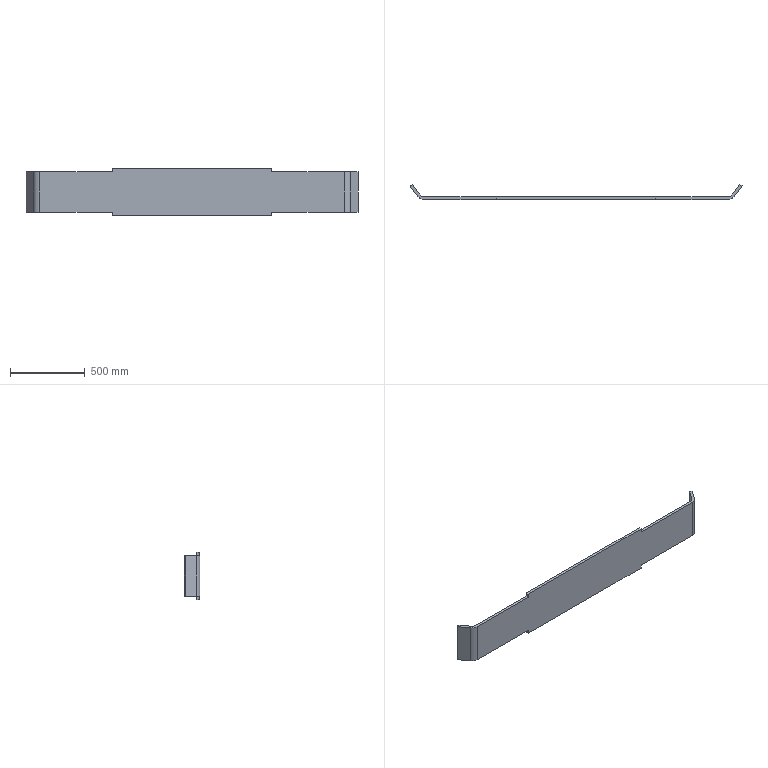Part | NX | features 前连杆 2 | 1 solid | 22 faces | box 2216 x 103.15 x 320 mm | volume 12312626 mm3 | plane 18 | cylinder 4 | commonest cylinder face diameters 60 x2 96.74 x2
STEP:
#1=CARTESIAN_POINT('',(-191.209,-83.211,25.));
#2=VERTEX_POINT('',#1);
#3=CARTESIAN_POINT('',(-243.821,-10.798,25.));
#4=VERTEX_POINT('',#3);
#5=CARTESIAN_POINT('',(957.045,-1663.648,25.));
#6=DIRECTION('',(-0.5878,0.809,0.));
#7=VECTOR('',#6,1000.);
#8=LINE('',#5,#7);
#9=EDGE_CURVE('',#2,#4,#8,.T.);
#10=ORIENTED_EDGE('',*,*,#9,.F.);
#11=CARTESIAN_POINT('',(-191.209,-83.211,295.));
#12=VERTEX_POINT('',#11);
#13=CARTESIAN_POINT('',(-191.209,-83.211,320.));
#14=DIRECTION('',(0.,0.,-1.));
#15=VECTOR('',#14,1000.);
#16=LINE('',#13,#15);
#17=EDGE_CURVE('',#12,#2,#16,.T.);
#18=ORIENTED_EDGE('',*,*,#17,.F.);
#19=CARTESIAN_POINT('',(-243.821,-10.798,295.));
#20=VERTEX_POINT('',#19);
#21=CARTESIAN_POINT('',(957.045,-1663.648,295.));
#22=DIRECTION('',(0.5878,-0.809,0.));
#23=VECTOR('',#22,1000.);
#24=LINE('',#21,#23);
#25=EDGE_CURVE('',#20,#12,#24,.T.);
#26=ORIENTED_EDGE('',*,*,#25,.F.);
#27=CARTESIAN_POINT('',(-243.821,-10.798,320.));
#28=DIRECTION('',(0.,0.,-1.));
#29=VECTOR('',#28,1000.);
#30=LINE('',#27,#29);
#31=EDGE_CURVE('',#20,#4,#30,.T.);
#32=ORIENTED_EDGE('',*,*,#31,.T.);
#33=EDGE_LOOP('',(#10,#18,#26,#32));
#34=FACE_BOUND('',#33,.T.);
#35=CARTESIAN_POINT('',(957.045,-1663.648,320.));
#36=DIRECTION('',(-0.809,-0.5878,0.));
#37=DIRECTION('',(0.5878,-0.809,0.));
#38=AXIS2_PLACEMENT_3D('',#35,#36,#37);
#39=PLANE('',#38);
#40=ADVANCED_FACE('',(#34),#39,.T.);
#41=ORIENTED_EDGE('',*,*,#17,.T.);
#42=CARTESIAN_POINT('',(-152.077,-103.15,25.));
#43=VERTEX_POINT('',#42);
#44=CARTESIAN_POINT('',(-152.077,-54.78,25.));
#45=DIRECTION('',(0.,0.,1.));
#46=DIRECTION('',(1.,0.,0.));
#47=AXIS2_PLACEMENT_3D('',#44,#45,#46);
#48=CIRCLE('',#47,48.37);
#49=EDGE_CURVE('',#2,#43,#48,.T.);
#50=ORIENTED_EDGE('',*,*,#49,.T.);
#51=CARTESIAN_POINT('',(-152.077,-103.15,295.));
#52=VERTEX_POINT('',#51);
#53=CARTESIAN_POINT('',(-152.077,-103.15,320.));
#54=DIRECTION('',(0.,0.,-1.));
#55=VECTOR('',#54,1000.);
#56=LINE('',#53,#55);
#57=EDGE_CURVE('',#52,#43,#56,.T.);
#58=ORIENTED_EDGE('',*,*,#57,.F.);
#59=CARTESIAN_POINT('',(-152.077,-54.78,295.));
#60=DIRECTION('',(0.,0.,-1.));
#61=DIRECTION('',(-1.,0.,0.));
#62=AXIS2_PLACEMENT_3D('',#59,#60,#61);
#63=CIRCLE('',#62,48.37);
#64=EDGE_CURVE('',#52,#12,#63,.T.);
#65=ORIENTED_EDGE('',*,*,#64,.T.);
#66=EDGE_LOOP('',(#41,#50,#58,#65));
#67=FACE_BOUND('',#66,.T.);
#68=CARTESIAN_POINT('',(-152.077,-54.78,320.));
#69=DIRECTION('',(0.,0.,-1.));
#70=DIRECTION('',(-1.,0.,0.));
#71=AXIS2_PLACEMENT_3D('',#68,#69,#70);
#72=CYLINDRICAL_SURFACE('',#71,48.37);
#73=ADVANCED_FACE('',(#67),#72,.T.);
#74=CARTESIAN_POINT('',(331.828,-103.15,25.));
#75=VERTEX_POINT('',#74);
#76=CARTESIAN_POINT('',(864.127,-103.15,25.));
#77=DIRECTION('',(1.,0.,0.));
#78=VECTOR('',#77,1000.);
#79=LINE('',#76,#78);
#80=EDGE_CURVE('',#43,#75,#79,.T.);
#81=ORIENTED_EDGE('',*,*,#80,.T.);
#82=CARTESIAN_POINT('',(331.828,-103.15,0.));
#83=VERTEX_POINT('',#82);
#84=CARTESIAN_POINT('',(331.828,-103.15,320.));
#85=DIRECTION('',(0.,0.,-1.));
#86=VECTOR('',#85,1000.);
#87=LINE('',#84,#86);
#88=EDGE_CURVE('',#75,#83,#87,.T.);
#89=ORIENTED_EDGE('',*,*,#88,.T.);
#90=CARTESIAN_POINT('',(1396.426,-103.15,0.));
#91=VERTEX_POINT('',#90);
#92=CARTESIAN_POINT('',(864.127,-103.15,0.));
#93=DIRECTION('',(1.,0.,0.));
#94=VECTOR('',#93,1000.);
#95=LINE('',#92,#94);
#96=EDGE_CURVE('',#83,#91,#95,.T.);
#97=ORIENTED_EDGE('',*,*,#96,.T.);
#98=CARTESIAN_POINT('',(1396.426,-103.15,25.));
#99=VERTEX_POINT('',#98);
#100=CARTESIAN_POINT('',(1396.426,-103.15,320.));
#101=DIRECTION('',(0.,0.,1.));
#102=VECTOR('',#101,1000.);
#103=LINE('',#100,#102);
#104=EDGE_CURVE('',#91,#99,#103,.T.);
#105=ORIENTED_EDGE('',*,*,#104,.T.);
#106=CARTESIAN_POINT('',(1880.331,-103.15,25.));
#107=VERTEX_POINT('',#106);
#108=CARTESIAN_POINT('',(864.127,-103.15,25.));
#109=DIRECTION('',(1.,0.,0.));
#110=VECTOR('',#109,1000.);
#111=LINE('',#108,#110);
#112=EDGE_CURVE('',#99,#107,#111,.T.);
#113=ORIENTED_EDGE('',*,*,#112,.T.);
#114=CARTESIAN_POINT('',(1880.331,-103.15,295.));
#115=VERTEX_POINT('',#114);
#116=CARTESIAN_POINT('',(1880.331,-103.15,320.));
#117=DIRECTION('',(0.,0.,-1.));
#118=VECTOR('',#117,1000.);
#119=LINE('',#116,#118);
#120=EDGE_CURVE('',#115,#107,#119,.T.);
#121=ORIENTED_EDGE('',*,*,#120,.F.);
#122=CARTESIAN_POINT('',(1396.426,-103.15,295.));
#123=VERTEX_POINT('',#122);
#124=CARTESIAN_POINT('',(864.127,-103.15,295.));
#125=DIRECTION('',(-1.,0.,0.));
#126=VECTOR('',#125,1000.);
#127=LINE('',#124,#126);
#128=EDGE_CURVE('',#115,#123,#127,.T.);
#129=ORIENTED_EDGE('',*,*,#128,.T.);
#130=CARTESIAN_POINT('',(1396.426,-103.15,320.));
#131=VERTEX_POINT('',#130);
#132=CARTESIAN_POINT('',(1396.426,-103.15,320.));
#133=DIRECTION('',(0.,0.,1.));
#134=VECTOR('',#133,1000.);
#135=LINE('',#132,#134);
#136=EDGE_CURVE('',#123,#131,#135,.T.);
#137=ORIENTED_EDGE('',*,*,#136,.T.);
#138=CARTESIAN_POINT('',(331.828,-103.15,320.));
#139=VERTEX_POINT('',#138);
#140=CARTESIAN_POINT('',(864.127,-103.15,320.));
#141=DIRECTION('',(1.,0.,0.));
#142=VECTOR('',#141,1000.);
#143=LINE('',#140,#142);
#144=EDGE_CURVE('',#139,#131,#143,.T.);
#145=ORIENTED_EDGE('',*,*,#144,.F.);
#146=CARTESIAN_POINT('',(331.828,-103.15,295.));
#147=VERTEX_POINT('',#146);
#148=CARTESIAN_POINT('',(331.828,-103.15,320.));
#149=DIRECTION('',(0.,0.,-1.));
#150=VECTOR('',#149,1000.);
#151=LINE('',#148,#150);
#152=EDGE_CURVE('',#139,#147,#151,.T.);
#153=ORIENTED_EDGE('',*,*,#152,.T.);
#154=CARTESIAN_POINT('',(864.127,-103.15,295.));
#155=DIRECTION('',(-1.,0.,0.));
#156=VECTOR('',#155,1000.);
#157=LINE('',#154,#156);
#158=EDGE_CURVE('',#147,#52,#157,.T.);
#159=ORIENTED_EDGE('',*,*,#158,.T.);
#160=ORIENTED_EDGE('',*,*,#57,.T.);
#161=EDGE_LOOP('',(#81,#89,#97,#105,#113,#121,#129,#137,#145,#153,#159,#160));
#162=FACE_BOUND('',#161,.T.);
#163=CARTESIAN_POINT('',(864.127,-103.15,320.));
#164=DIRECTION('',(0.,1.,0.));
#165=DIRECTION('',(-1.,0.,0.));
#166=AXIS2_PLACEMENT_3D('',#163,#164,#165);
#167=PLANE('',#166);
#168=ADVANCED_FACE('',(#162),#167,.F.);
#169=CARTESIAN_POINT('',(1919.464,-83.211,25.));
#170=VERTEX_POINT('',#169);
#171=CARTESIAN_POINT('',(1880.331,-54.78,25.));
#172=DIRECTION('',(0.,0.,1.));
#173=DIRECTION('',(1.,0.,0.));
#174=AXIS2_PLACEMENT_3D('',#171,#172,#173);
#175=CIRCLE('',#174,48.37);
#176=EDGE_CURVE('',#170,#107,#175,.F.);
#177=ORIENTED_EDGE('',*,*,#176,.F.);
#178=CARTESIAN_POINT('',(1919.464,-83.211,295.));
#179=VERTEX_POINT('',#178);
#180=CARTESIAN_POINT('',(1919.464,-83.211,320.));
#181=DIRECTION('',(0.,0.,-1.));
#182=VECTOR('',#181,1000.);
#183=LINE('',#180,#182);
#184=EDGE_CURVE('',#179,#170,#183,.T.);
#185=ORIENTED_EDGE('',*,*,#184,.F.);
#186=CARTESIAN_POINT('',(1880.331,-54.78,295.));
#187=DIRECTION('',(0.,0.,-1.));
#188=DIRECTION('',(-1.,0.,0.));
#189=AXIS2_PLACEMENT_3D('',#186,#187,#188);
#190=CIRCLE('',#189,48.37);
#191=EDGE_CURVE('',#115,#179,#190,.F.);
#192=ORIENTED_EDGE('',*,*,#191,.F.);
#193=ORIENTED_EDGE('',*,*,#120,.T.);
#194=EDGE_LOOP('',(#177,#185,#192,#193));
#195=FACE_BOUND('',#194,.T.);
#196=CARTESIAN_POINT('',(1880.331,-54.78,320.));
#197=DIRECTION('',(0.,0.,-1.));
#198=DIRECTION('',(-1.,0.,0.));
#199=AXIS2_PLACEMENT_3D('',#196,#197,#198);
#200=CYLINDRICAL_SURFACE('',#199,48.37);
#201=ADVANCED_FACE('',(#195),#200,.T.);
#202=ORIENTED_EDGE('',*,*,#184,.T.);
#203=CARTESIAN_POINT('',(1972.075,-10.798,25.));
#204=VERTEX_POINT('',#203);
#205=CARTESIAN_POINT('',(771.209,-1663.648,25.));
#206=DIRECTION('',(0.5878,0.809,0.));
#207=VECTOR('',#206,1000.);
#208=LINE('',#205,#207);
#209=EDGE_CURVE('',#170,#204,#208,.T.);
#210=ORIENTED_EDGE('',*,*,#209,.T.);
#211=CARTESIAN_POINT('',(1972.075,-10.798,295.));
#212=VERTEX_POINT('',#211);
#213=CARTESIAN_POINT('',(1972.075,-10.798,320.));
#214=DIRECTION('',(0.,0.,-1.));
#215=VECTOR('',#214,1000.);
#216=LINE('',#213,#215);
#217=EDGE_CURVE('',#212,#204,#216,.T.);
#218=ORIENTED_EDGE('',*,*,#217,.F.);
#219=CARTESIAN_POINT('',(771.209,-1663.648,295.));
#220=DIRECTION('',(-0.5878,-0.809,0.));
#221=VECTOR('',#220,1000.);
#222=LINE('',#219,#221);
#223=EDGE_CURVE('',#212,#179,#222,.T.);
#224=ORIENTED_EDGE('',*,*,#223,.T.);
#225=EDGE_LOOP('',(#202,#210,#218,#224));
#226=FACE_BOUND('',#225,.T.);
#227=CARTESIAN_POINT('',(771.209,-1663.648,320.));
#228=DIRECTION('',(-0.809,0.5878,0.));
#229=DIRECTION('',(-0.5878,-0.809,0.));
#230=AXIS2_PLACEMENT_3D('',#227,#228,#229);
#231=PLANE('',#230);
#232=ADVANCED_FACE('',(#226),#231,.F.);
#233=ORIENTED_EDGE('',*,*,#217,.T.);
#234=CARTESIAN_POINT('',(1957.213,0.,25.));
#235=VERTEX_POINT('',#234);
#236=CARTESIAN_POINT('',(2064.993,-78.307,25.));
#237=DIRECTION('',(-0.809,0.5878,0.));
#238=VECTOR('',#237,1000.);
#239=LINE('',#236,#238);
#240=EDGE_CURVE('',#204,#235,#239,.T.);
#241=ORIENTED_EDGE('',*,*,#240,.T.);
#242=CARTESIAN_POINT('',(1957.213,0.,295.));
#243=VERTEX_POINT('',#242);
#244=CARTESIAN_POINT('',(1957.213,0.,320.));
#245=DIRECTION('',(0.,0.,-1.));
#246=VECTOR('',#245,1000.);
#247=LINE('',#244,#246);
#248=EDGE_CURVE('',#243,#235,#247,.T.);
#249=ORIENTED_EDGE('',*,*,#248,.F.);
#250=CARTESIAN_POINT('',(2064.993,-78.307,295.));
#251=DIRECTION('',(0.809,-0.5878,0.));
#252=VECTOR('',#251,1000.);
#253=LINE('',#250,#252);
#254=EDGE_CURVE('',#243,#212,#253,.T.);
#255=ORIENTED_EDGE('',*,*,#254,.T.);
#256=EDGE_LOOP('',(#233,#241,#249,#255));
#257=FACE_BOUND('',#256,.T.);
#258=CARTESIAN_POINT('',(2064.993,-78.307,320.));
#259=DIRECTION('',(-0.5878,-0.809,0.));
#260=DIRECTION('',(0.809,-0.5878,0.));
#261=AXIS2_PLACEMENT_3D('',#258,#259,#260);
#262=PLANE('',#261);
#263=ADVANCED_FACE('',(#257),#262,.F.);
#264=CARTESIAN_POINT('',(1904.602,-72.414,25.));
#265=VERTEX_POINT('',#264);
#266=CARTESIAN_POINT('',(756.347,-1652.851,25.));
#267=DIRECTION('',(0.5878,0.809,0.));
#268=VECTOR('',#267,1000.);
#269=LINE('',#266,#268);
#270=EDGE_CURVE('',#265,#235,#269,.T.);
#271=ORIENTED_EDGE('',*,*,#270,.F.);
#272=CARTESIAN_POINT('',(1904.602,-72.414,295.));
#273=VERTEX_POINT('',#272);
#274=CARTESIAN_POINT('',(1904.602,-72.414,320.));
#275=DIRECTION('',(0.,0.,-1.));
#276=VECTOR('',#275,1000.);
#277=LINE('',#274,#276);
#278=EDGE_CURVE('',#273,#265,#277,.T.);
#279=ORIENTED_EDGE('',*,*,#278,.F.);
#280=CARTESIAN_POINT('',(756.347,-1652.851,295.));
#281=DIRECTION('',(-0.5878,-0.809,0.));
#282=VECTOR('',#281,1000.);
#283=LINE('',#280,#282);
#284=EDGE_CURVE('',#243,#273,#283,.T.);
#285=ORIENTED_EDGE('',*,*,#284,.F.);
#286=ORIENTED_EDGE('',*,*,#248,.T.);
#287=EDGE_LOOP('',(#271,#279,#285,#286));
#288=FACE_BOUND('',#287,.T.);
#289=CARTESIAN_POINT('',(756.347,-1652.851,320.));
#290=DIRECTION('',(-0.809,0.5878,0.));
#291=DIRECTION('',(-0.5878,-0.809,0.));
#292=AXIS2_PLACEMENT_3D('',#289,#290,#291);
#293=PLANE('',#292);
#294=ADVANCED_FACE('',(#288),#293,.T.);
#295=ORIENTED_EDGE('',*,*,#278,.T.);
#296=CARTESIAN_POINT('',(1880.331,-84.78,25.));
#297=VERTEX_POINT('',#296);
#298=CARTESIAN_POINT('',(1880.331,-54.78,25.));
#299=DIRECTION('',(0.,0.,1.));
#300=DIRECTION('',(1.,0.,0.));
#301=AXIS2_PLACEMENT_3D('',#298,#299,#300);
#302=CIRCLE('',#301,30.);
#303=EDGE_CURVE('',#265,#297,#302,.F.);
#304=ORIENTED_EDGE('',*,*,#303,.T.);
#305=CARTESIAN_POINT('',(1880.331,-84.78,295.));
#306=VERTEX_POINT('',#305);
#307=CARTESIAN_POINT('',(1880.331,-84.78,320.));
#308=DIRECTION('',(0.,0.,-1.));
#309=VECTOR('',#308,1000.);
#310=LINE('',#307,#309);
#311=EDGE_CURVE('',#306,#297,#310,.T.);
#312=ORIENTED_EDGE('',*,*,#311,.F.);
#313=CARTESIAN_POINT('',(1880.331,-54.78,295.));
#314=DIRECTION('',(0.,0.,-1.));
#315=DIRECTION('',(-1.,0.,0.));
#316=AXIS2_PLACEMENT_3D('',#313,#314,#315);
#317=CIRCLE('',#316,30.);
#318=EDGE_CURVE('',#306,#273,#317,.F.);
#319=ORIENTED_EDGE('',*,*,#318,.T.);
#320=EDGE_LOOP('',(#295,#304,#312,#319));
#321=FACE_BOUND('',#320,.T.);
#322=CARTESIAN_POINT('',(1880.331,-54.78,320.));
#323=DIRECTION('',(0.,0.,-1.));
#324=DIRECTION('',(-1.,0.,0.));
#325=AXIS2_PLACEMENT_3D('',#322,#323,#324);
#326=CYLINDRICAL_SURFACE('',#325,30.);
#327=ADVANCED_FACE('',(#321),#326,.F.);
#328=CARTESIAN_POINT('',(331.828,-84.78,25.));
#329=VERTEX_POINT('',#328);
#330=CARTESIAN_POINT('',(331.828,-84.78,0.));
#331=VERTEX_POINT('',#330);
#332=CARTESIAN_POINT('',(331.828,-84.78,320.));
#333=DIRECTION('',(0.,0.,-1.));
#334=VECTOR('',#333,1000.);
#335=LINE('',#332,#334);
#336=EDGE_CURVE('',#329,#331,#335,.T.);
#337=ORIENTED_EDGE('',*,*,#336,.F.);
#338=CARTESIAN_POINT('',(-152.077,-84.78,25.));
#339=VERTEX_POINT('',#338);
#340=CARTESIAN_POINT('',(864.127,-84.78,25.));
#341=DIRECTION('',(1.,0.,0.));
#342=VECTOR('',#341,1000.);
#343=LINE('',#340,#342);
#344=EDGE_CURVE('',#339,#329,#343,.T.);
#345=ORIENTED_EDGE('',*,*,#344,.F.);
#346=CARTESIAN_POINT('',(-152.077,-84.78,295.));
#347=VERTEX_POINT('',#346);
#348=CARTESIAN_POINT('',(-152.077,-84.78,320.));
#349=DIRECTION('',(0.,0.,-1.));
#350=VECTOR('',#349,1000.);
#351=LINE('',#348,#350);
#352=EDGE_CURVE('',#347,#339,#351,.T.);
#353=ORIENTED_EDGE('',*,*,#352,.F.);
#354=CARTESIAN_POINT('',(331.828,-84.78,295.));
#355=VERTEX_POINT('',#354);
#356=CARTESIAN_POINT('',(864.127,-84.78,295.));
#357=DIRECTION('',(-1.,0.,0.));
#358=VECTOR('',#357,1000.);
#359=LINE('',#356,#358);
#360=EDGE_CURVE('',#355,#347,#359,.T.);
#361=ORIENTED_EDGE('',*,*,#360,.F.);
#362=CARTESIAN_POINT('',(331.828,-84.78,320.));
#363=VERTEX_POINT('',#362);
#364=CARTESIAN_POINT('',(331.828,-84.78,320.));
#365=DIRECTION('',(0.,0.,-1.));
#366=VECTOR('',#365,1000.);
#367=LINE('',#364,#366);
#368=EDGE_CURVE('',#363,#355,#367,.T.);
#369=ORIENTED_EDGE('',*,*,#368,.F.);
#370=CARTESIAN_POINT('',(1396.426,-84.78,320.));
#371=VERTEX_POINT('',#370);
#372=CARTESIAN_POINT('',(864.127,-84.78,320.));
#373=DIRECTION('',(1.,0.,0.));
#374=VECTOR('',#373,1000.);
#375=LINE('',#372,#374);
#376=EDGE_CURVE('',#363,#371,#375,.T.);
#377=ORIENTED_EDGE('',*,*,#376,.T.);
#378=CARTESIAN_POINT('',(1396.426,-84.78,295.));
#379=VERTEX_POINT('',#378);
#380=CARTESIAN_POINT('',(1396.426,-84.78,320.));
#381=DIRECTION('',(0.,0.,1.));
#382=VECTOR('',#381,1000.);
#383=LINE('',#380,#382);
#384=EDGE_CURVE('',#379,#371,#383,.T.);
#385=ORIENTED_EDGE('',*,*,#384,.F.);
#386=CARTESIAN_POINT('',(864.127,-84.78,295.));
#387=DIRECTION('',(-1.,0.,0.));
#388=VECTOR('',#387,1000.);
#389=LINE('',#386,#388);
#390=EDGE_CURVE('',#306,#379,#389,.T.);
#391=ORIENTED_EDGE('',*,*,#390,.F.);
#392=ORIENTED_EDGE('',*,*,#311,.T.);
#393=CARTESIAN_POINT('',(1396.426,-84.78,25.));
#394=VERTEX_POINT('',#393);
#395=CARTESIAN_POINT('',(864.127,-84.78,25.));
#396=DIRECTION('',(1.,0.,0.));
#397=VECTOR('',#396,1000.);
#398=LINE('',#395,#397);
#399=EDGE_CURVE('',#394,#297,#398,.T.);
#400=ORIENTED_EDGE('',*,*,#399,.F.);
#401=CARTESIAN_POINT('',(1396.426,-84.78,0.));
#402=VERTEX_POINT('',#401);
#403=CARTESIAN_POINT('',(1396.426,-84.78,320.));
#404=DIRECTION('',(0.,0.,1.));
#405=VECTOR('',#404,1000.);
#406=LINE('',#403,#405);
#407=EDGE_CURVE('',#402,#394,#406,.T.);
#408=ORIENTED_EDGE('',*,*,#407,.F.);
#409=CARTESIAN_POINT('',(864.127,-84.78,0.));
#410=DIRECTION('',(1.,0.,0.));
#411=VECTOR('',#410,1000.);
#412=LINE('',#409,#411);
#413=EDGE_CURVE('',#331,#402,#412,.T.);
#414=ORIENTED_EDGE('',*,*,#413,.F.);
#415=EDGE_LOOP('',(#337,#345,#353,#361,#369,#377,#385,#391,#392,#400,#408,#414));
#416=FACE_BOUND('',#415,.T.);
#417=CARTESIAN_POINT('',(864.127,-84.78,320.));
#418=DIRECTION('',(0.,1.,0.));
#419=DIRECTION('',(0.,0.,1.));
#420=AXIS2_PLACEMENT_3D('',#417,#418,#419);
#421=PLANE('',#420);
#422=ADVANCED_FACE('',(#416),#421,.T.);
#423=CARTESIAN_POINT('',(-176.348,-72.414,25.));
#424=VERTEX_POINT('',#423);
#425=CARTESIAN_POINT('',(-152.077,-54.78,25.));
#426=DIRECTION('',(0.,0.,1.));
#427=DIRECTION('',(1.,0.,0.));
#428=AXIS2_PLACEMENT_3D('',#425,#426,#427);
#429=CIRCLE('',#428,30.);
#430=EDGE_CURVE('',#424,#339,#429,.T.);
#431=ORIENTED_EDGE('',*,*,#430,.F.);
#432=CARTESIAN_POINT('',(-176.348,-72.414,295.));
#433=VERTEX_POINT('',#432);
#434=CARTESIAN_POINT('',(-176.348,-72.414,320.));
#435=DIRECTION('',(0.,0.,-1.));
#436=VECTOR('',#435,1000.);
#437=LINE('',#434,#436);
#438=EDGE_CURVE('',#433,#424,#437,.T.);
#439=ORIENTED_EDGE('',*,*,#438,.F.);
#440=CARTESIAN_POINT('',(-152.077,-54.78,295.));
#441=DIRECTION('',(0.,0.,-1.));
#442=DIRECTION('',(-1.,0.,0.));
#443=AXIS2_PLACEMENT_3D('',#440,#441,#442);
#444=CIRCLE('',#443,30.);
#445=EDGE_CURVE('',#347,#433,#444,.T.);
#446=ORIENTED_EDGE('',*,*,#445,.F.);
#447=ORIENTED_EDGE('',*,*,#352,.T.);
#448=EDGE_LOOP('',(#431,#439,#446,#447));
#449=FACE_BOUND('',#448,.T.);
#450=CARTESIAN_POINT('',(-152.077,-54.78,320.));
#451=DIRECTION('',(0.,0.,-1.));
#452=DIRECTION('',(-1.,0.,0.));
#453=AXIS2_PLACEMENT_3D('',#450,#451,#452);
#454=CYLINDRICAL_SURFACE('',#453,30.);
#455=ADVANCED_FACE('',(#449),#454,.F.);
#456=ORIENTED_EDGE('',*,*,#438,.T.);
#457=CARTESIAN_POINT('',(-228.959,0.,25.));
#458=VERTEX_POINT('',#457);
#459=CARTESIAN_POINT('',(971.907,-1652.851,25.));
#460=DIRECTION('',(-0.5878,0.809,0.));
#461=VECTOR('',#460,1000.);
#462=LINE('',#459,#461);
#463=EDGE_CURVE('',#424,#458,#462,.T.);
#464=ORIENTED_EDGE('',*,*,#463,.T.);
#465=CARTESIAN_POINT('',(-228.959,0.,295.));
#466=VERTEX_POINT('',#465);
#467=CARTESIAN_POINT('',(-228.959,0.,320.));
#468=DIRECTION('',(0.,0.,-1.));
#469=VECTOR('',#468,1000.);
#470=LINE('',#467,#469);
#471=EDGE_CURVE('',#466,#458,#470,.T.);
#472=ORIENTED_EDGE('',*,*,#471,.F.);
#473=CARTESIAN_POINT('',(971.907,-1652.851,295.));
#474=DIRECTION('',(0.5878,-0.809,0.));
#475=VECTOR('',#474,1000.);
#476=LINE('',#473,#475);
#477=EDGE_CURVE('',#466,#433,#476,.T.);
#478=ORIENTED_EDGE('',*,*,#477,.T.);
#479=EDGE_LOOP('',(#456,#464,#472,#478));
#480=FACE_BOUND('',#479,.T.);
#481=CARTESIAN_POINT('',(971.907,-1652.851,320.));
#482=DIRECTION('',(-0.809,-0.5878,0.));
#483=DIRECTION('',(0.5878,-0.809,0.));
#484=AXIS2_PLACEMENT_3D('',#481,#482,#483);
#485=PLANE('',#484);
#486=ADVANCED_FACE('',(#480),#485,.F.);
#487=CARTESIAN_POINT('',(-336.739,-78.307,25.));
#488=DIRECTION('',(0.809,0.5878,0.));
#489=VECTOR('',#488,1000.);
#490=LINE('',#487,#489);
#491=EDGE_CURVE('',#4,#458,#490,.T.);
#492=ORIENTED_EDGE('',*,*,#491,.F.);
#493=ORIENTED_EDGE('',*,*,#31,.F.);
#494=CARTESIAN_POINT('',(-336.739,-78.307,295.));
#495=DIRECTION('',(-0.809,-0.5878,0.));
#496=VECTOR('',#495,1000.);
#497=LINE('',#494,#496);
#498=EDGE_CURVE('',#466,#20,#497,.T.);
#499=ORIENTED_EDGE('',*,*,#498,.F.);
#500=ORIENTED_EDGE('',*,*,#471,.T.);
#501=EDGE_LOOP('',(#492,#493,#499,#500));
#502=FACE_BOUND('',#501,.T.);
#503=CARTESIAN_POINT('',(-336.739,-78.307,320.));
#504=DIRECTION('',(-0.5878,0.809,0.));
#505=DIRECTION('',(-0.809,-0.5878,0.));
#506=AXIS2_PLACEMENT_3D('',#503,#504,#505);
#507=PLANE('',#506);
#508=ADVANCED_FACE('',(#502),#507,.T.);
#509=CARTESIAN_POINT('',(331.828,-1731.157,320.));
#510=DIRECTION('',(0.,1.,0.));
#511=VECTOR('',#510,1000.);
#512=LINE('',#509,#511);
#513=EDGE_CURVE('',#139,#363,#512,.T.);
#514=ORIENTED_EDGE('',*,*,#513,.F.);
#515=ORIENTED_EDGE('',*,*,#144,.T.);
#516=CARTESIAN_POINT('',(1396.426,-1731.157,320.));
#517=DIRECTION('',(0.,-1.,0.));
#518=VECTOR('',#517,1000.);
#519=LINE('',#516,#518);
#520=EDGE_CURVE('',#371,#131,#519,.T.);
#521=ORIENTED_EDGE('',*,*,#520,.F.);
#522=ORIENTED_EDGE('',*,*,#376,.F.);
#523=EDGE_LOOP('',(#514,#515,#521,#522));
#524=FACE_BOUND('',#523,.T.);
#525=CARTESIAN_POINT('',(864.127,-1731.157,320.));
#526=DIRECTION('',(0.,0.,1.));
#527=DIRECTION('',(1.,0.,0.));
#528=AXIS2_PLACEMENT_3D('',#525,#526,#527);
#529=PLANE('',#528);
#530=ADVANCED_FACE('',(#524),#529,.T.);
#531=ORIENTED_EDGE('',*,*,#96,.F.);
#532=CARTESIAN_POINT('',(331.828,-1731.157,0.));
#533=DIRECTION('',(0.,1.,0.));
#534=VECTOR('',#533,1000.);
#535=LINE('',#532,#534);
#536=EDGE_CURVE('',#83,#331,#535,.T.);
#537=ORIENTED_EDGE('',*,*,#536,.T.);
#538=ORIENTED_EDGE('',*,*,#413,.T.);
#539=CARTESIAN_POINT('',(1396.426,-1731.157,0.));
#540=DIRECTION('',(0.,-1.,0.));
#541=VECTOR('',#540,1000.);
#542=LINE('',#539,#541);
#543=EDGE_CURVE('',#402,#91,#542,.T.);
#544=ORIENTED_EDGE('',*,*,#543,.T.);
#545=EDGE_LOOP('',(#531,#537,#538,#544));
#546=FACE_BOUND('',#545,.T.);
#547=CARTESIAN_POINT('',(864.127,-1731.157,0.));
#548=DIRECTION('',(0.,0.,1.));
#549=DIRECTION('',(1.,0.,0.));
#550=AXIS2_PLACEMENT_3D('',#547,#548,#549);
#551=PLANE('',#550);
#552=ADVANCED_FACE('',(#546),#551,.F.);
#553=CARTESIAN_POINT('',(1396.426,-160.,25.));
#554=DIRECTION('',(0.,1.,0.));
#555=VECTOR('',#554,1000.);
#556=LINE('',#553,#555);
#557=EDGE_CURVE('',#99,#394,#556,.T.);
#558=ORIENTED_EDGE('',*,*,#557,.T.);
#559=ORIENTED_EDGE('',*,*,#399,.T.);
#560=ORIENTED_EDGE('',*,*,#303,.F.);
#561=ORIENTED_EDGE('',*,*,#270,.T.);
#562=ORIENTED_EDGE('',*,*,#240,.F.);
#563=ORIENTED_EDGE('',*,*,#209,.F.);
#564=ORIENTED_EDGE('',*,*,#176,.T.);
#565=ORIENTED_EDGE('',*,*,#112,.F.);
#566=EDGE_LOOP('',(#558,#559,#560,#561,#562,#563,#564,#565));
#567=FACE_BOUND('',#566,.T.);
#568=CARTESIAN_POINT('',(1972.075,-160.,25.));
#569=DIRECTION('',(0.,0.,1.));
#570=DIRECTION('',(1.,0.,0.));
#571=AXIS2_PLACEMENT_3D('',#568,#569,#570);
#572=PLANE('',#571);
#573=ADVANCED_FACE('',(#567),#572,.F.);
#574=ORIENTED_EDGE('',*,*,#543,.F.);
#575=ORIENTED_EDGE('',*,*,#407,.T.);
#576=ORIENTED_EDGE('',*,*,#557,.F.);
#577=ORIENTED_EDGE('',*,*,#104,.F.);
#578=EDGE_LOOP('',(#574,#575,#576,#577));
#579=FACE_BOUND('',#578,.T.);
#580=CARTESIAN_POINT('',(1396.426,-160.,0.));
#581=DIRECTION('',(-1.,0.,0.));
#582=DIRECTION('',(0.,-1.,0.));
#583=AXIS2_PLACEMENT_3D('',#580,#581,#582);
#584=PLANE('',#583);
#585=ADVANCED_FACE('',(#579),#584,.F.);
#586=ORIENTED_EDGE('',*,*,#49,.F.);
#587=ORIENTED_EDGE('',*,*,#9,.T.);
#588=ORIENTED_EDGE('',*,*,#491,.T.);
#589=ORIENTED_EDGE('',*,*,#463,.F.);
#590=ORIENTED_EDGE('',*,*,#430,.T.);
#591=ORIENTED_EDGE('',*,*,#344,.T.);
#592=CARTESIAN_POINT('',(331.828,-160.,25.));
#593=DIRECTION('',(0.,1.,0.));
#594=VECTOR('',#593,1000.);
#595=LINE('',#592,#594);
#596=EDGE_CURVE('',#75,#329,#595,.T.);
#597=ORIENTED_EDGE('',*,*,#596,.F.);
#598=ORIENTED_EDGE('',*,*,#80,.F.);
#599=EDGE_LOOP('',(#586,#587,#588,#589,#590,#591,#597,#598));
#600=FACE_BOUND('',#599,.T.);
#601=CARTESIAN_POINT('',(-243.821,-160.,25.));
#602=DIRECTION('',(0.,0.,1.));
#603=DIRECTION('',(1.,0.,0.));
#604=AXIS2_PLACEMENT_3D('',#601,#602,#603);
#605=PLANE('',#604);
#606=ADVANCED_FACE('',(#600),#605,.F.);
#607=ORIENTED_EDGE('',*,*,#596,.T.);
#608=ORIENTED_EDGE('',*,*,#336,.T.);
#609=ORIENTED_EDGE('',*,*,#536,.F.);
#610=ORIENTED_EDGE('',*,*,#88,.F.);
#611=EDGE_LOOP('',(#607,#608,#609,#610));
#612=FACE_BOUND('',#611,.T.);
#613=CARTESIAN_POINT('',(331.828,-160.,0.));
#614=DIRECTION('',(1.,0.,0.));
#615=DIRECTION('',(0.,1.,0.));
#616=AXIS2_PLACEMENT_3D('',#613,#614,#615);
#617=PLANE('',#616);
#618=ADVANCED_FACE('',(#612),#617,.F.);
#619=ORIENTED_EDGE('',*,*,#191,.T.);
#620=ORIENTED_EDGE('',*,*,#223,.F.);
#621=ORIENTED_EDGE('',*,*,#254,.F.);
#622=ORIENTED_EDGE('',*,*,#284,.T.);
#623=ORIENTED_EDGE('',*,*,#318,.F.);
#624=ORIENTED_EDGE('',*,*,#390,.T.);
#625=CARTESIAN_POINT('',(1396.426,-160.,295.));
#626=DIRECTION('',(0.,1.,0.));
#627=VECTOR('',#626,1000.);
#628=LINE('',#625,#627);
#629=EDGE_CURVE('',#123,#379,#628,.T.);
#630=ORIENTED_EDGE('',*,*,#629,.F.);
#631=ORIENTED_EDGE('',*,*,#128,.F.);
#632=EDGE_LOOP('',(#619,#620,#621,#622,#623,#624,#630,#631));
#633=FACE_BOUND('',#632,.T.);
#634=CARTESIAN_POINT('',(1972.075,-160.,295.));
#635=DIRECTION('',(0.,0.,-1.));
#636=DIRECTION('',(-1.,0.,0.));
#637=AXIS2_PLACEMENT_3D('',#634,#635,#636);
#638=PLANE('',#637);
#639=ADVANCED_FACE('',(#633),#638,.F.);
#640=ORIENTED_EDGE('',*,*,#629,.T.);
#641=ORIENTED_EDGE('',*,*,#384,.T.);
#642=ORIENTED_EDGE('',*,*,#520,.T.);
#643=ORIENTED_EDGE('',*,*,#136,.F.);
#644=EDGE_LOOP('',(#640,#641,#642,#643));
#645=FACE_BOUND('',#644,.T.);
#646=CARTESIAN_POINT('',(1396.426,-160.,320.));
#647=DIRECTION('',(-1.,0.,0.));
#648=DIRECTION('',(0.,-1.,0.));
#649=AXIS2_PLACEMENT_3D('',#646,#647,#648);
#650=PLANE('',#649);
#651=ADVANCED_FACE('',(#645),#650,.F.);
#652=CARTESIAN_POINT('',(331.828,-160.,295.));
#653=DIRECTION('',(0.,1.,0.));
#654=VECTOR('',#653,1000.);
#655=LINE('',#652,#654);
#656=EDGE_CURVE('',#147,#355,#655,.T.);
#657=ORIENTED_EDGE('',*,*,#656,.T.);
#658=ORIENTED_EDGE('',*,*,#360,.T.);
#659=ORIENTED_EDGE('',*,*,#445,.T.);
#660=ORIENTED_EDGE('',*,*,#477,.F.);
#661=ORIENTED_EDGE('',*,*,#498,.T.);
#662=ORIENTED_EDGE('',*,*,#25,.T.);
#663=ORIENTED_EDGE('',*,*,#64,.F.);
#664=ORIENTED_EDGE('',*,*,#158,.F.);
#665=EDGE_LOOP('',(#657,#658,#659,#660,#661,#662,#663,#664));
#666=FACE_BOUND('',#665,.T.);
#667=CARTESIAN_POINT('',(-243.821,-160.,295.));
#668=DIRECTION('',(0.,0.,-1.));
#669=DIRECTION('',(-1.,0.,0.));
#670=AXIS2_PLACEMENT_3D('',#667,#668,#669);
#671=PLANE('',#670);
#672=ADVANCED_FACE('',(#666),#671,.F.);
#673=ORIENTED_EDGE('',*,*,#513,.T.);
#674=ORIENTED_EDGE('',*,*,#368,.T.);
#675=ORIENTED_EDGE('',*,*,#656,.F.);
#676=ORIENTED_EDGE('',*,*,#152,.F.);
#677=EDGE_LOOP('',(#673,#674,#675,#676));
#678=FACE_BOUND('',#677,.T.);
#679=CARTESIAN_POINT('',(331.828,-160.,320.));
#680=DIRECTION('',(1.,0.,0.));
#681=DIRECTION('',(0.,1.,0.));
#682=AXIS2_PLACEMENT_3D('',#679,#680,#681);
#683=PLANE('',#682);
#684=ADVANCED_FACE('',(#678),#683,.F.);
#685=CLOSED_SHELL('',(#40,#73,#168,#201,#232,#263,#294,#327,#422,#455,#486,#508,#530,#552,#573,#585,#606,#618,#639,#651,#672,#684));
#686=MANIFOLD_SOLID_BREP('',#685);
#687=(LENGTH_UNIT()NAMED_UNIT(*)SI_UNIT(.MILLI.,.METRE.));
#688=UNCERTAINTY_MEASURE_WITH_UNIT(LENGTH_MEASURE(0.00001),#687,'','');
#689=(NAMED_UNIT(*)PLANE_ANGLE_UNIT()SI_UNIT($,.RADIAN.));
#690=(NAMED_UNIT(*)SI_UNIT($,.STERADIAN.)SOLID_ANGLE_UNIT());
#691=(GEOMETRIC_REPRESENTATION_CONTEXT(3)GLOBAL_UNCERTAINTY_ASSIGNED_CONTEXT((#688))GLOBAL_UNIT_ASSIGNED_CONTEXT((#687,#689,#690))REPRESENTATION_CONTEXT('',''));
#692=ADVANCED_BREP_SHAPE_REPRESENTATION('',(#686),#691);